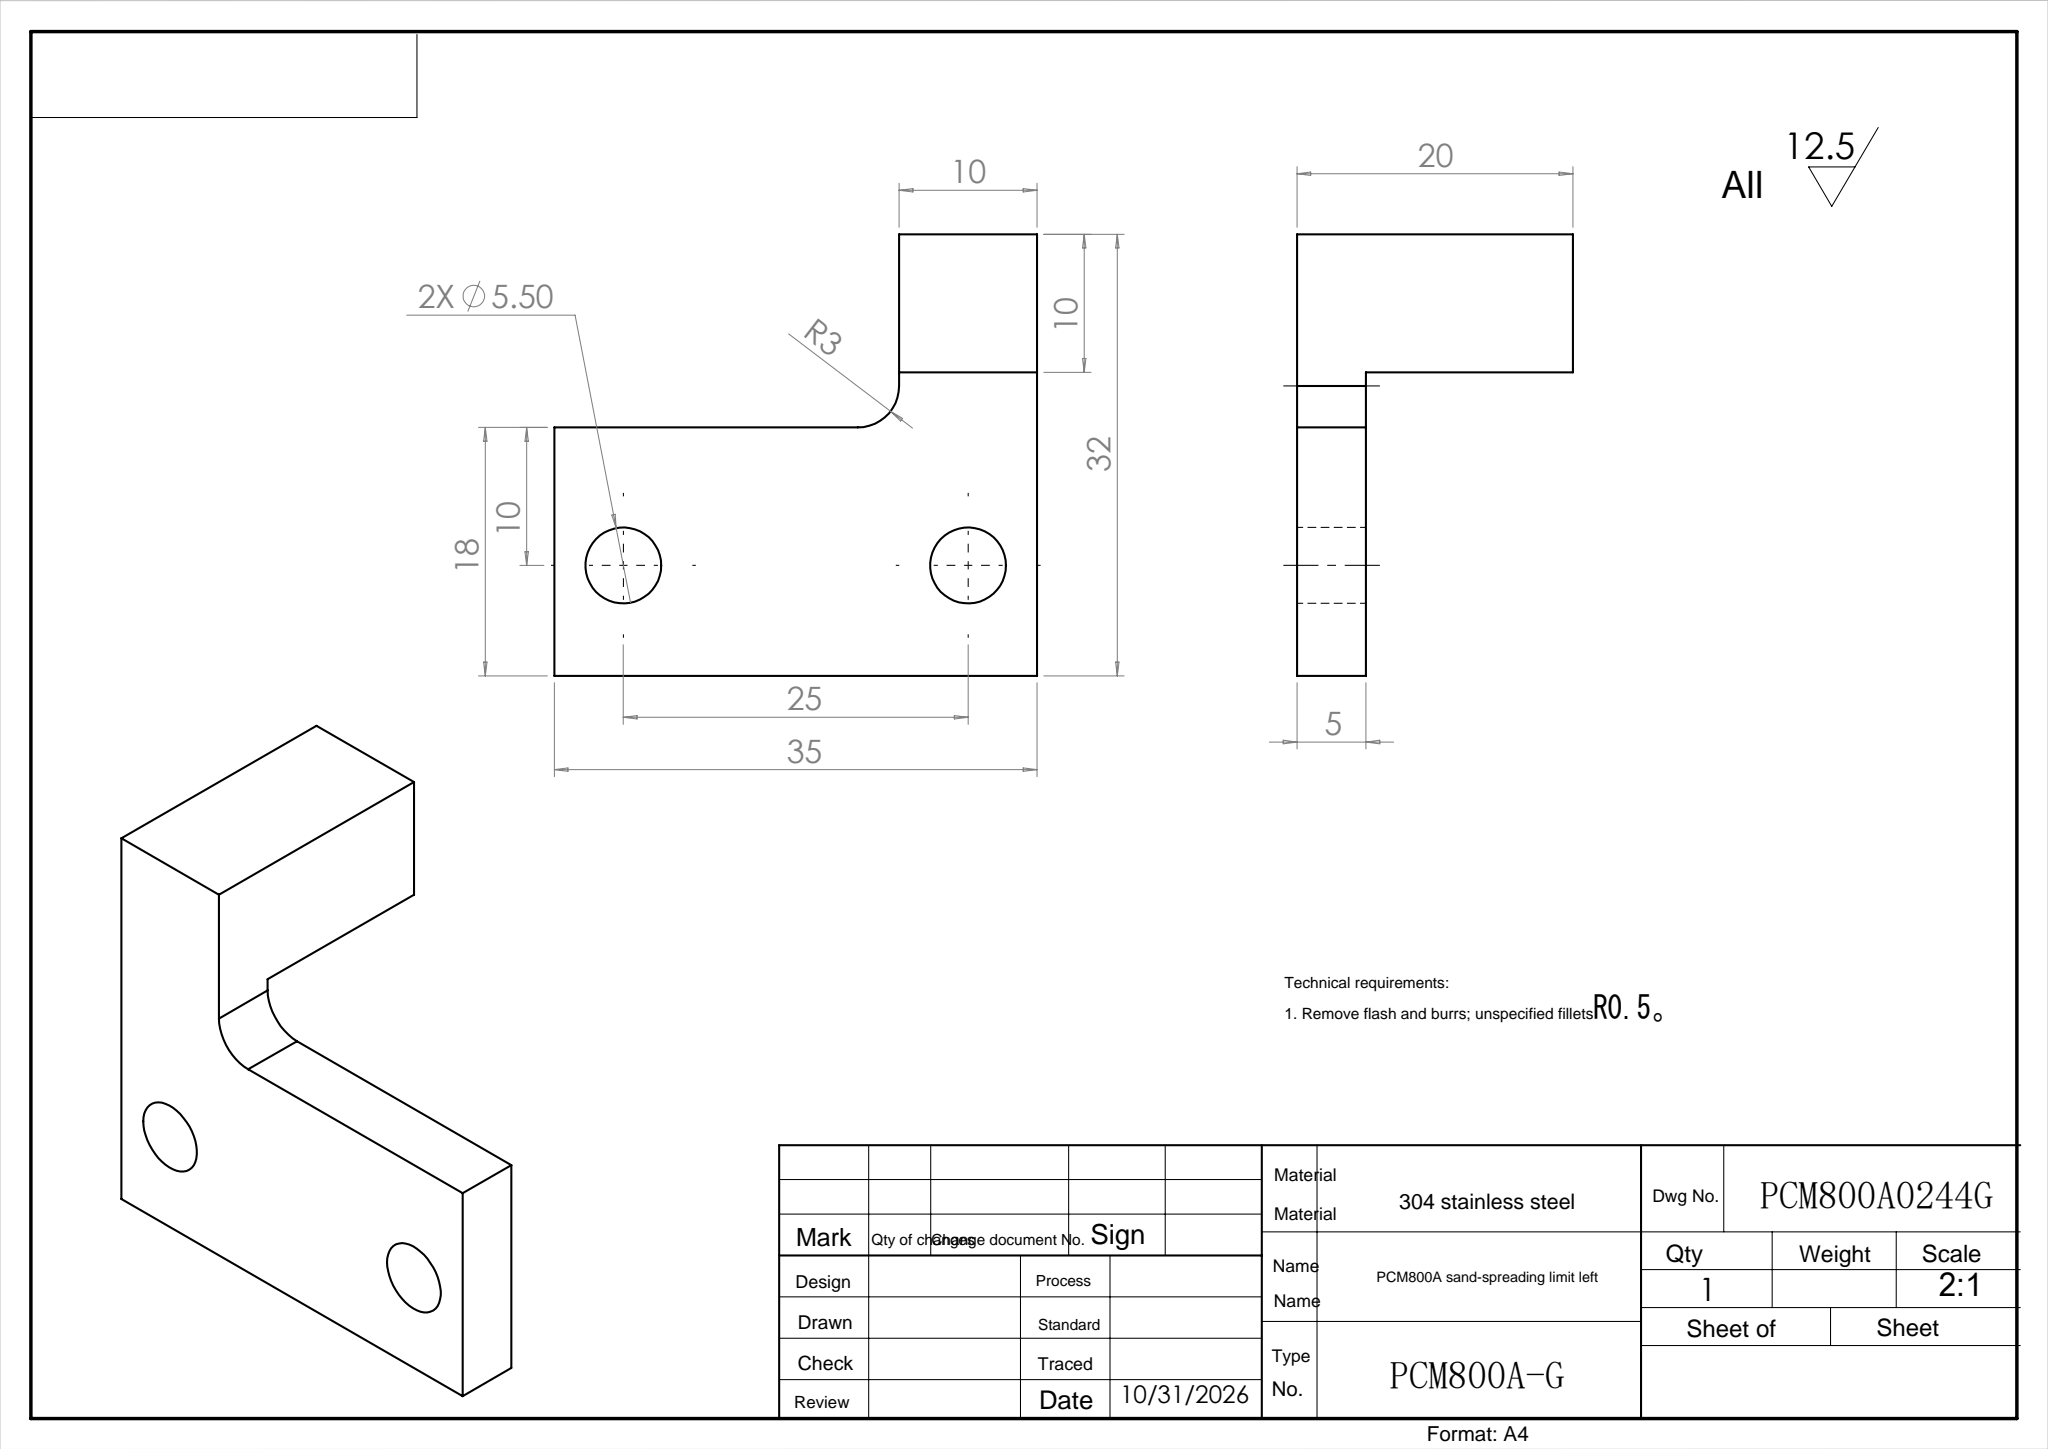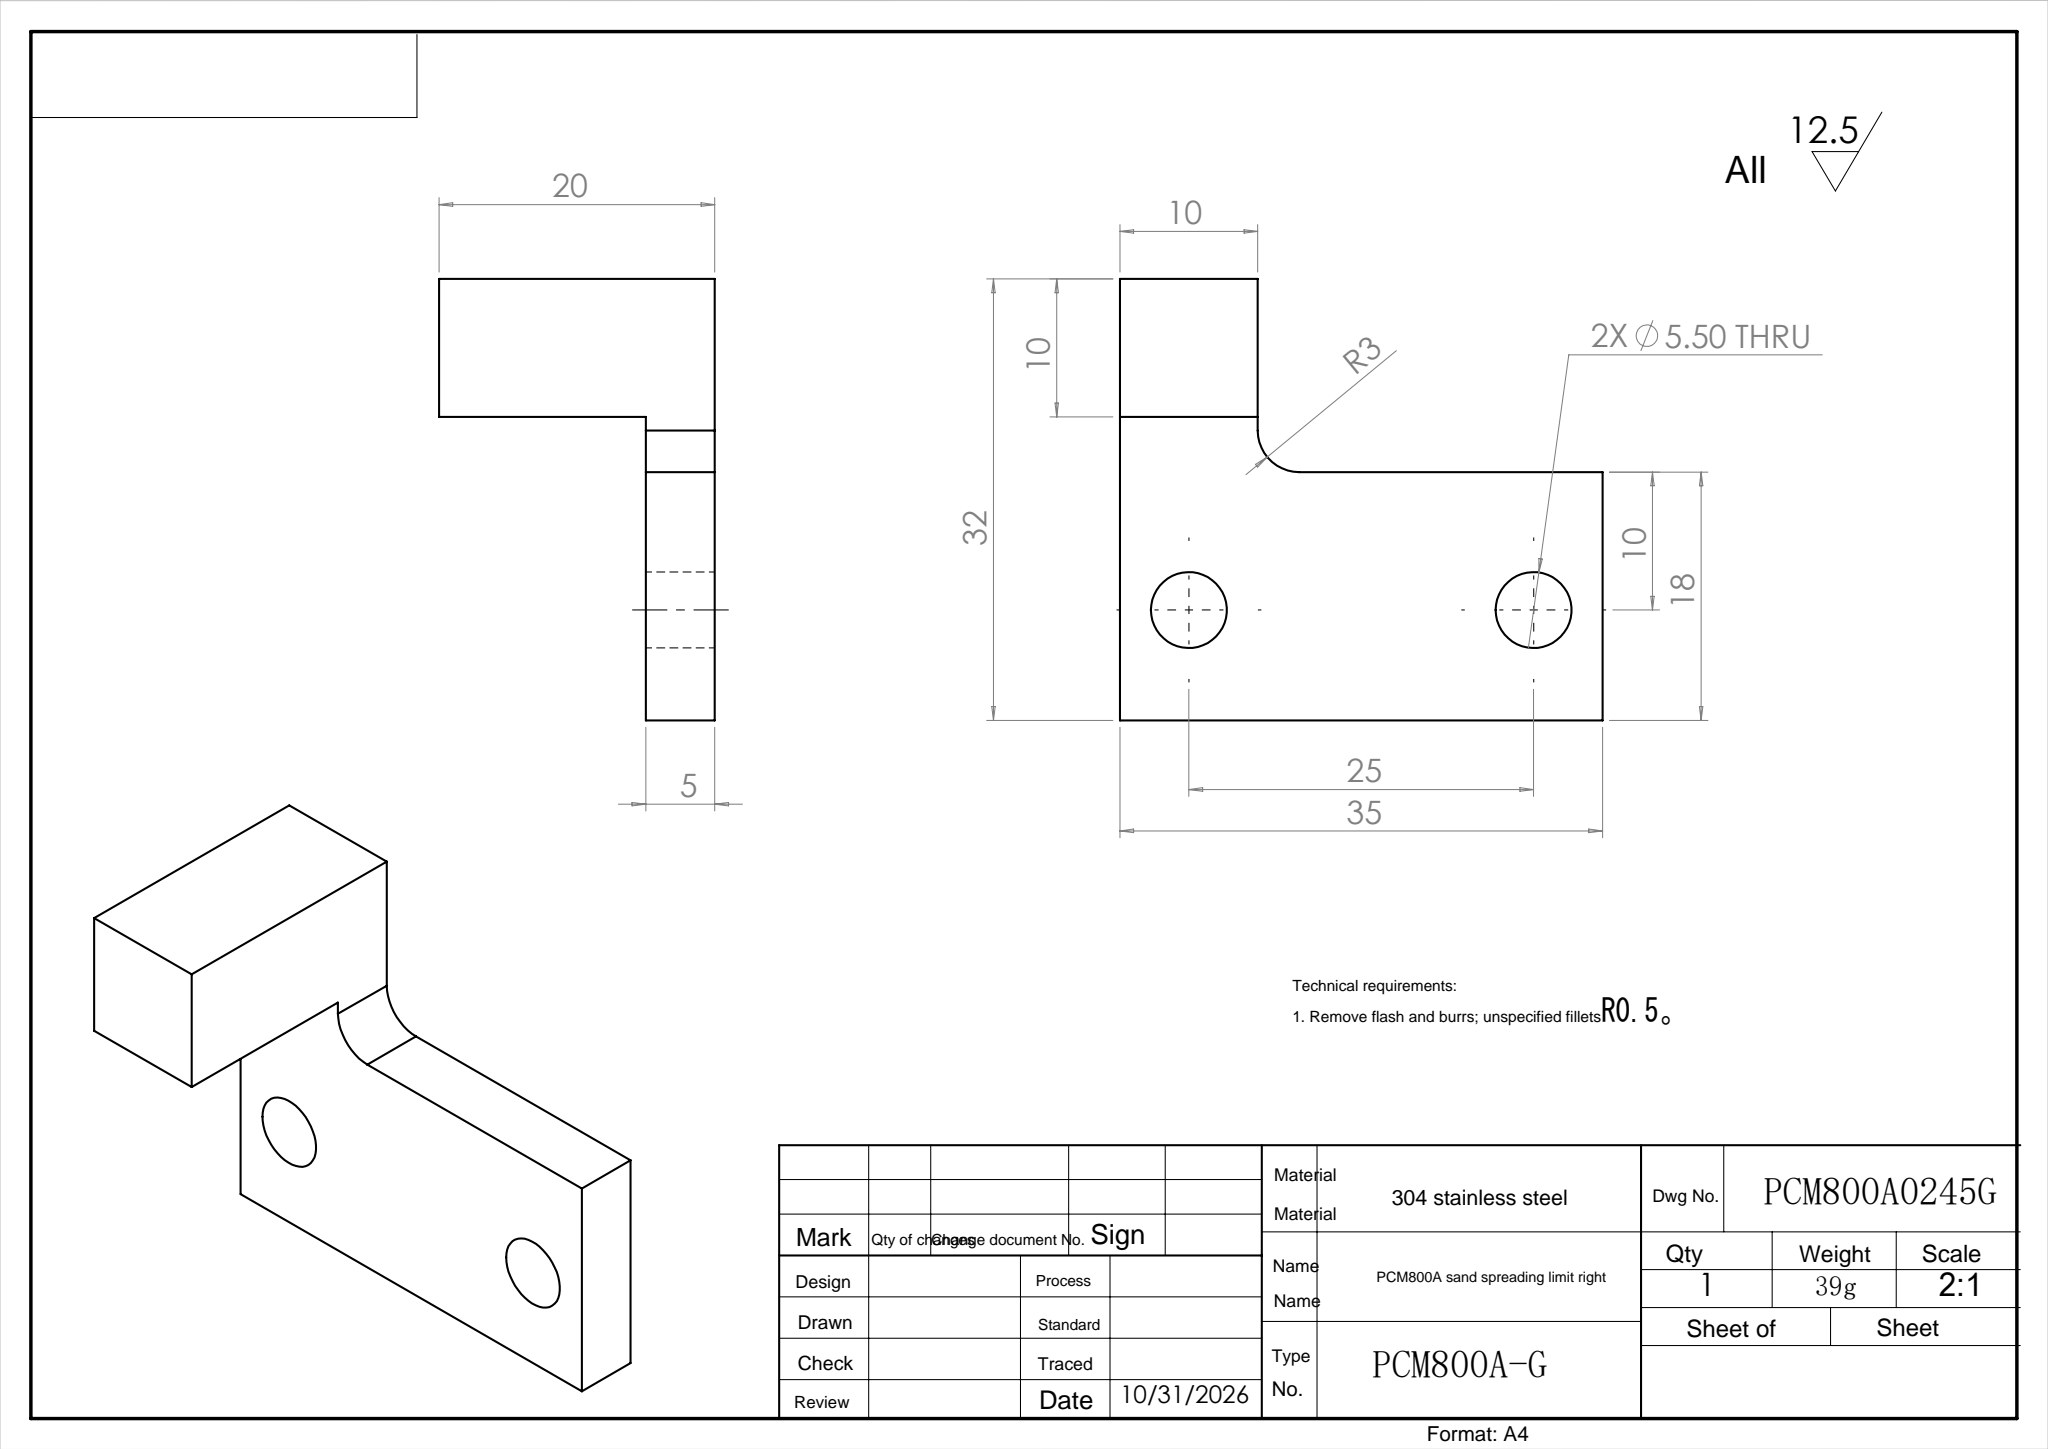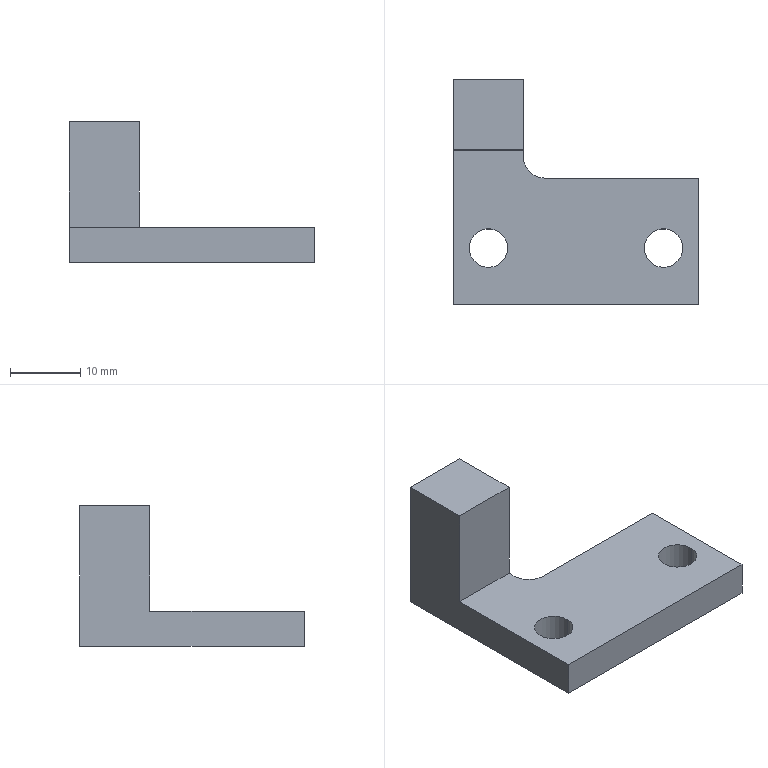Part | SolidWorks | features ICE 2, Extrusion 1 | 1 solid | 15 faces | box 35 x 32 x 20 mm | volume 5122 mm3 | plane 10 | cylinder 5 | commonest cylinder face diameters 5.5 x4 6 x1
STEP:
#1=CARTESIAN_POINT('',(7.75,8.,5.));
#2=VERTEX_POINT('',#1);
#3=CARTESIAN_POINT('',(2.25,8.,5.));
#4=VERTEX_POINT('',#3);
#5=CARTESIAN_POINT('',(5.,8.,5.));
#6=DIRECTION('',(0.,0.,-1.));
#7=DIRECTION('',(-1.,0.,0.));
#8=AXIS2_PLACEMENT_3D('',#5,#6,#7);
#9=CIRCLE('',#8,2.75);
#10=EDGE_CURVE('',#2,#4,#9,.T.);
#11=ORIENTED_EDGE('',*,*,#10,.F.);
#12=CARTESIAN_POINT('',(7.75,8.,0.));
#13=VERTEX_POINT('',#12);
#14=CARTESIAN_POINT('',(7.75,8.,20.));
#15=DIRECTION('',(0.,0.,-1.));
#16=VECTOR('',#15,1000.);
#17=LINE('',#14,#16);
#18=EDGE_CURVE('',#2,#13,#17,.T.);
#19=ORIENTED_EDGE('',*,*,#18,.T.);
#20=CARTESIAN_POINT('',(2.25,8.,0.));
#21=VERTEX_POINT('',#20);
#22=CARTESIAN_POINT('',(5.,8.,0.));
#23=DIRECTION('',(0.,0.,-1.));
#24=DIRECTION('',(-1.,0.,0.));
#25=AXIS2_PLACEMENT_3D('',#22,#23,#24);
#26=CIRCLE('',#25,2.75);
#27=EDGE_CURVE('',#13,#21,#26,.T.);
#28=ORIENTED_EDGE('',*,*,#27,.T.);
#29=CARTESIAN_POINT('',(2.25,8.,20.));
#30=DIRECTION('',(0.,0.,-1.));
#31=VECTOR('',#30,1000.);
#32=LINE('',#29,#31);
#33=EDGE_CURVE('',#4,#21,#32,.T.);
#34=ORIENTED_EDGE('',*,*,#33,.F.);
#35=EDGE_LOOP('',(#11,#19,#28,#34));
#36=FACE_OUTER_BOUND('',#35,.T.);
#37=CARTESIAN_POINT('',(5.,8.,20.));
#38=DIRECTION('',(0.,0.,-1.));
#39=DIRECTION('',(-1.,0.,0.));
#40=AXIS2_PLACEMENT_3D('',#37,#38,#39);
#41=CYLINDRICAL_SURFACE('',#40,2.75);
#42=ADVANCED_FACE('',(#36),#41,.F.);
#43=CARTESIAN_POINT('',(32.75,8.,5.));
#44=VERTEX_POINT('',#43);
#45=CARTESIAN_POINT('',(27.25,8.,5.));
#46=VERTEX_POINT('',#45);
#47=CARTESIAN_POINT('',(30.,8.,5.));
#48=DIRECTION('',(0.,0.,-1.));
#49=DIRECTION('',(-1.,0.,0.));
#50=AXIS2_PLACEMENT_3D('',#47,#48,#49);
#51=CIRCLE('',#50,2.75);
#52=EDGE_CURVE('',#44,#46,#51,.T.);
#53=ORIENTED_EDGE('',*,*,#52,.F.);
#54=CARTESIAN_POINT('',(32.75,8.,0.));
#55=VERTEX_POINT('',#54);
#56=CARTESIAN_POINT('',(32.75,8.,20.));
#57=DIRECTION('',(0.,0.,-1.));
#58=VECTOR('',#57,1000.);
#59=LINE('',#56,#58);
#60=EDGE_CURVE('',#44,#55,#59,.T.);
#61=ORIENTED_EDGE('',*,*,#60,.T.);
#62=CARTESIAN_POINT('',(27.25,8.,0.));
#63=VERTEX_POINT('',#62);
#64=CARTESIAN_POINT('',(30.,8.,0.));
#65=DIRECTION('',(0.,0.,-1.));
#66=DIRECTION('',(-1.,0.,0.));
#67=AXIS2_PLACEMENT_3D('',#64,#65,#66);
#68=CIRCLE('',#67,2.75);
#69=EDGE_CURVE('',#55,#63,#68,.T.);
#70=ORIENTED_EDGE('',*,*,#69,.T.);
#71=CARTESIAN_POINT('',(27.25,8.,20.));
#72=DIRECTION('',(0.,0.,-1.));
#73=VECTOR('',#72,1000.);
#74=LINE('',#71,#73);
#75=EDGE_CURVE('',#46,#63,#74,.T.);
#76=ORIENTED_EDGE('',*,*,#75,.F.);
#77=EDGE_LOOP('',(#53,#61,#70,#76));
#78=FACE_OUTER_BOUND('',#77,.T.);
#79=CARTESIAN_POINT('',(30.,8.,20.));
#80=DIRECTION('',(0.,0.,-1.));
#81=DIRECTION('',(-1.,0.,0.));
#82=AXIS2_PLACEMENT_3D('',#79,#80,#81);
#83=CYLINDRICAL_SURFACE('',#82,2.75);
#84=ADVANCED_FACE('',(#78),#83,.F.);
#85=CARTESIAN_POINT('',(0.,32.,0.));
#86=VERTEX_POINT('',#85);
#87=CARTESIAN_POINT('',(0.,0.,0.));
#88=VERTEX_POINT('',#87);
#89=CARTESIAN_POINT('',(0.,0.,0.));
#90=DIRECTION('',(0.,-1.,0.));
#91=VECTOR('',#90,1000.);
#92=LINE('',#89,#91);
#93=EDGE_CURVE('',#86,#88,#92,.T.);
#94=ORIENTED_EDGE('',*,*,#93,.T.);
#95=CARTESIAN_POINT('',(0.,0.,5.));
#96=VERTEX_POINT('',#95);
#97=CARTESIAN_POINT('',(0.,0.,5.));
#98=DIRECTION('',(0.,0.,-1.));
#99=VECTOR('',#98,1000.);
#100=LINE('',#97,#99);
#101=EDGE_CURVE('',#96,#88,#100,.T.);
#102=ORIENTED_EDGE('',*,*,#101,.F.);
#103=CARTESIAN_POINT('',(0.,22.,5.));
#104=VERTEX_POINT('',#103);
#105=CARTESIAN_POINT('',(0.,0.,5.));
#106=DIRECTION('',(0.,-1.,0.));
#107=VECTOR('',#106,1000.);
#108=LINE('',#105,#107);
#109=EDGE_CURVE('',#104,#96,#108,.T.);
#110=ORIENTED_EDGE('',*,*,#109,.F.);
#111=CARTESIAN_POINT('',(0.,22.,20.));
#112=VERTEX_POINT('',#111);
#113=CARTESIAN_POINT('',(0.,22.,20.));
#114=DIRECTION('',(0.,0.,-1.));
#115=VECTOR('',#114,1000.);
#116=LINE('',#113,#115);
#117=EDGE_CURVE('',#112,#104,#116,.T.);
#118=ORIENTED_EDGE('',*,*,#117,.F.);
#119=CARTESIAN_POINT('',(0.,32.,20.));
#120=VERTEX_POINT('',#119);
#121=CARTESIAN_POINT('',(0.,22.,20.));
#122=DIRECTION('',(0.,1.,0.));
#123=VECTOR('',#122,1000.);
#124=LINE('',#121,#123);
#125=EDGE_CURVE('',#112,#120,#124,.T.);
#126=ORIENTED_EDGE('',*,*,#125,.T.);
#127=CARTESIAN_POINT('',(0.,32.,20.));
#128=DIRECTION('',(0.,0.,-1.));
#129=VECTOR('',#128,1000.);
#130=LINE('',#127,#129);
#131=EDGE_CURVE('',#120,#86,#130,.T.);
#132=ORIENTED_EDGE('',*,*,#131,.T.);
#133=EDGE_LOOP('',(#94,#102,#110,#118,#126,#132));
#134=FACE_OUTER_BOUND('',#133,.T.);
#135=CARTESIAN_POINT('',(0.,0.,5.));
#136=DIRECTION('',(1.,0.,0.));
#137=DIRECTION('',(0.,0.,-1.));
#138=AXIS2_PLACEMENT_3D('',#135,#136,#137);
#139=PLANE('',#138);
#140=ADVANCED_FACE('',(#134),#139,.F.);
#141=CARTESIAN_POINT('',(35.,0.,0.));
#142=VERTEX_POINT('',#141);
#143=CARTESIAN_POINT('',(0.,0.,0.));
#144=DIRECTION('',(1.,0.,0.));
#145=VECTOR('',#144,1000.);
#146=LINE('',#143,#145);
#147=EDGE_CURVE('',#88,#142,#146,.T.);
#148=ORIENTED_EDGE('',*,*,#147,.T.);
#149=CARTESIAN_POINT('',(35.,0.,5.));
#150=VERTEX_POINT('',#149);
#151=CARTESIAN_POINT('',(35.,0.,5.));
#152=DIRECTION('',(0.,0.,-1.));
#153=VECTOR('',#152,1000.);
#154=LINE('',#151,#153);
#155=EDGE_CURVE('',#150,#142,#154,.T.);
#156=ORIENTED_EDGE('',*,*,#155,.F.);
#157=CARTESIAN_POINT('',(0.,0.,5.));
#158=DIRECTION('',(1.,0.,0.));
#159=VECTOR('',#158,1000.);
#160=LINE('',#157,#159);
#161=EDGE_CURVE('',#96,#150,#160,.T.);
#162=ORIENTED_EDGE('',*,*,#161,.F.);
#163=ORIENTED_EDGE('',*,*,#101,.T.);
#164=EDGE_LOOP('',(#148,#156,#162,#163));
#165=FACE_OUTER_BOUND('',#164,.T.);
#166=CARTESIAN_POINT('',(0.,0.,5.));
#167=DIRECTION('',(0.,1.,0.));
#168=DIRECTION('',(0.,0.,1.));
#169=AXIS2_PLACEMENT_3D('',#166,#167,#168);
#170=PLANE('',#169);
#171=ADVANCED_FACE('',(#165),#170,.F.);
#172=CARTESIAN_POINT('',(35.,18.,0.));
#173=VERTEX_POINT('',#172);
#174=CARTESIAN_POINT('',(35.,0.,0.));
#175=DIRECTION('',(0.,1.,0.));
#176=VECTOR('',#175,1000.);
#177=LINE('',#174,#176);
#178=EDGE_CURVE('',#142,#173,#177,.T.);
#179=ORIENTED_EDGE('',*,*,#178,.T.);
#180=CARTESIAN_POINT('',(35.,18.,5.));
#181=VERTEX_POINT('',#180);
#182=CARTESIAN_POINT('',(35.,18.,5.));
#183=DIRECTION('',(0.,0.,-1.));
#184=VECTOR('',#183,1000.);
#185=LINE('',#182,#184);
#186=EDGE_CURVE('',#181,#173,#185,.T.);
#187=ORIENTED_EDGE('',*,*,#186,.F.);
#188=CARTESIAN_POINT('',(35.,0.,5.));
#189=DIRECTION('',(0.,1.,0.));
#190=VECTOR('',#189,1000.);
#191=LINE('',#188,#190);
#192=EDGE_CURVE('',#150,#181,#191,.T.);
#193=ORIENTED_EDGE('',*,*,#192,.F.);
#194=ORIENTED_EDGE('',*,*,#155,.T.);
#195=EDGE_LOOP('',(#179,#187,#193,#194));
#196=FACE_OUTER_BOUND('',#195,.T.);
#197=CARTESIAN_POINT('',(35.,0.,5.));
#198=DIRECTION('',(-1.,0.,0.));
#199=DIRECTION('',(0.,0.,1.));
#200=AXIS2_PLACEMENT_3D('',#197,#198,#199);
#201=PLANE('',#200);
#202=ADVANCED_FACE('',(#196),#201,.F.);
#203=CARTESIAN_POINT('',(13.,18.,0.));
#204=VERTEX_POINT('',#203);
#205=CARTESIAN_POINT('',(13.,18.,0.));
#206=DIRECTION('',(-1.,0.,0.));
#207=VECTOR('',#206,1000.);
#208=LINE('',#205,#207);
#209=EDGE_CURVE('',#173,#204,#208,.T.);
#210=ORIENTED_EDGE('',*,*,#209,.T.);
#211=CARTESIAN_POINT('',(13.,18.,5.));
#212=VERTEX_POINT('',#211);
#213=CARTESIAN_POINT('',(13.,18.,5.));
#214=DIRECTION('',(0.,0.,-1.));
#215=VECTOR('',#214,1000.);
#216=LINE('',#213,#215);
#217=EDGE_CURVE('',#212,#204,#216,.T.);
#218=ORIENTED_EDGE('',*,*,#217,.F.);
#219=CARTESIAN_POINT('',(13.,18.,5.));
#220=DIRECTION('',(-1.,0.,0.));
#221=VECTOR('',#220,1000.);
#222=LINE('',#219,#221);
#223=EDGE_CURVE('',#181,#212,#222,.T.);
#224=ORIENTED_EDGE('',*,*,#223,.F.);
#225=ORIENTED_EDGE('',*,*,#186,.T.);
#226=EDGE_LOOP('',(#210,#218,#224,#225));
#227=FACE_OUTER_BOUND('',#226,.T.);
#228=CARTESIAN_POINT('',(13.,18.,5.));
#229=DIRECTION('',(0.,-1.,0.));
#230=DIRECTION('',(0.,0.,-1.));
#231=AXIS2_PLACEMENT_3D('',#228,#229,#230);
#232=PLANE('',#231);
#233=ADVANCED_FACE('',(#227),#232,.F.);
#234=CARTESIAN_POINT('',(10.,21.,0.));
#235=VERTEX_POINT('',#234);
#236=CARTESIAN_POINT('',(13.,21.,0.));
#237=DIRECTION('',(0.,0.,-1.));
#238=DIRECTION('',(-1.,0.,0.));
#239=AXIS2_PLACEMENT_3D('',#236,#237,#238);
#240=CIRCLE('',#239,3.);
#241=EDGE_CURVE('',#204,#235,#240,.T.);
#242=ORIENTED_EDGE('',*,*,#241,.T.);
#243=CARTESIAN_POINT('',(10.,21.,5.));
#244=VERTEX_POINT('',#243);
#245=CARTESIAN_POINT('',(10.,21.,5.));
#246=DIRECTION('',(0.,0.,-1.));
#247=VECTOR('',#246,1000.);
#248=LINE('',#245,#247);
#249=EDGE_CURVE('',#244,#235,#248,.T.);
#250=ORIENTED_EDGE('',*,*,#249,.F.);
#251=CARTESIAN_POINT('',(13.,21.,5.));
#252=DIRECTION('',(0.,0.,-1.));
#253=DIRECTION('',(-1.,0.,0.));
#254=AXIS2_PLACEMENT_3D('',#251,#252,#253);
#255=CIRCLE('',#254,3.);
#256=EDGE_CURVE('',#212,#244,#255,.T.);
#257=ORIENTED_EDGE('',*,*,#256,.F.);
#258=ORIENTED_EDGE('',*,*,#217,.T.);
#259=EDGE_LOOP('',(#242,#250,#257,#258));
#260=FACE_OUTER_BOUND('',#259,.T.);
#261=CARTESIAN_POINT('',(13.,21.,5.));
#262=DIRECTION('',(0.,0.,-1.));
#263=DIRECTION('',(-1.,0.,0.));
#264=AXIS2_PLACEMENT_3D('',#261,#262,#263);
#265=CYLINDRICAL_SURFACE('',#264,3.);
#266=ADVANCED_FACE('',(#260),#265,.F.);
#267=CARTESIAN_POINT('',(10.,32.,0.));
#268=VERTEX_POINT('',#267);
#269=CARTESIAN_POINT('',(10.,21.,0.));
#270=DIRECTION('',(0.,1.,0.));
#271=VECTOR('',#270,1000.);
#272=LINE('',#269,#271);
#273=EDGE_CURVE('',#235,#268,#272,.T.);
#274=ORIENTED_EDGE('',*,*,#273,.T.);
#275=CARTESIAN_POINT('',(10.,32.,20.));
#276=VERTEX_POINT('',#275);
#277=CARTESIAN_POINT('',(10.,32.,20.));
#278=DIRECTION('',(0.,0.,-1.));
#279=VECTOR('',#278,1000.);
#280=LINE('',#277,#279);
#281=EDGE_CURVE('',#276,#268,#280,.T.);
#282=ORIENTED_EDGE('',*,*,#281,.F.);
#283=CARTESIAN_POINT('',(10.,22.,20.));
#284=VERTEX_POINT('',#283);
#285=CARTESIAN_POINT('',(10.,22.,20.));
#286=DIRECTION('',(0.,-1.,0.));
#287=VECTOR('',#286,1000.);
#288=LINE('',#285,#287);
#289=EDGE_CURVE('',#276,#284,#288,.T.);
#290=ORIENTED_EDGE('',*,*,#289,.T.);
#291=CARTESIAN_POINT('',(10.,22.,5.));
#292=VERTEX_POINT('',#291);
#293=CARTESIAN_POINT('',(10.,22.,20.));
#294=DIRECTION('',(0.,0.,-1.));
#295=VECTOR('',#294,1000.);
#296=LINE('',#293,#295);
#297=EDGE_CURVE('',#284,#292,#296,.T.);
#298=ORIENTED_EDGE('',*,*,#297,.T.);
#299=CARTESIAN_POINT('',(10.,21.,5.));
#300=DIRECTION('',(0.,1.,0.));
#301=VECTOR('',#300,1000.);
#302=LINE('',#299,#301);
#303=EDGE_CURVE('',#244,#292,#302,.T.);
#304=ORIENTED_EDGE('',*,*,#303,.F.);
#305=ORIENTED_EDGE('',*,*,#249,.T.);
#306=EDGE_LOOP('',(#274,#282,#290,#298,#304,#305));
#307=FACE_OUTER_BOUND('',#306,.T.);
#308=CARTESIAN_POINT('',(10.,21.,5.));
#309=DIRECTION('',(-1.,0.,0.));
#310=DIRECTION('',(0.,-1.,0.));
#311=AXIS2_PLACEMENT_3D('',#308,#309,#310);
#312=PLANE('',#311);
#313=ADVANCED_FACE('',(#307),#312,.F.);
#314=CARTESIAN_POINT('',(5.,8.,5.));
#315=DIRECTION('',(0.,0.,-1.));
#316=DIRECTION('',(-1.,0.,0.));
#317=AXIS2_PLACEMENT_3D('',#314,#315,#316);
#318=CIRCLE('',#317,2.75);
#319=EDGE_CURVE('',#4,#2,#318,.T.);
#320=ORIENTED_EDGE('',*,*,#319,.T.);
#321=ORIENTED_EDGE('',*,*,#10,.T.);
#322=EDGE_LOOP('',(#320,#321));
#323=FACE_BOUND('',#322,.T.);
#324=CARTESIAN_POINT('',(30.,8.,5.));
#325=DIRECTION('',(0.,0.,-1.));
#326=DIRECTION('',(-1.,0.,0.));
#327=AXIS2_PLACEMENT_3D('',#324,#325,#326);
#328=CIRCLE('',#327,2.75);
#329=EDGE_CURVE('',#46,#44,#328,.T.);
#330=ORIENTED_EDGE('',*,*,#329,.T.);
#331=ORIENTED_EDGE('',*,*,#52,.T.);
#332=EDGE_LOOP('',(#330,#331));
#333=FACE_BOUND('',#332,.T.);
#334=ORIENTED_EDGE('',*,*,#109,.T.);
#335=ORIENTED_EDGE('',*,*,#161,.T.);
#336=ORIENTED_EDGE('',*,*,#192,.T.);
#337=ORIENTED_EDGE('',*,*,#223,.T.);
#338=ORIENTED_EDGE('',*,*,#256,.T.);
#339=ORIENTED_EDGE('',*,*,#303,.T.);
#340=CARTESIAN_POINT('',(0.,22.,5.));
#341=DIRECTION('',(-1.,0.,0.));
#342=VECTOR('',#341,1000.);
#343=LINE('',#340,#342);
#344=EDGE_CURVE('',#292,#104,#343,.T.);
#345=ORIENTED_EDGE('',*,*,#344,.T.);
#346=EDGE_LOOP('',(#334,#335,#336,#337,#338,#339,#345));
#347=FACE_OUTER_BOUND('',#346,.T.);
#348=CARTESIAN_POINT('',(13.,21.,5.));
#349=DIRECTION('',(0.,0.,-1.));
#350=DIRECTION('',(-1.,0.,0.));
#351=AXIS2_PLACEMENT_3D('',#348,#349,#350);
#352=PLANE('',#351);
#353=ADVANCED_FACE('',(#323,#333,#347),#352,.F.);
#354=CARTESIAN_POINT('',(5.,8.,0.));
#355=DIRECTION('',(0.,0.,-1.));
#356=DIRECTION('',(-1.,0.,0.));
#357=AXIS2_PLACEMENT_3D('',#354,#355,#356);
#358=CIRCLE('',#357,2.75);
#359=EDGE_CURVE('',#21,#13,#358,.T.);
#360=ORIENTED_EDGE('',*,*,#359,.F.);
#361=ORIENTED_EDGE('',*,*,#27,.F.);
#362=EDGE_LOOP('',(#360,#361));
#363=FACE_BOUND('',#362,.T.);
#364=CARTESIAN_POINT('',(30.,8.,0.));
#365=DIRECTION('',(0.,0.,-1.));
#366=DIRECTION('',(-1.,0.,0.));
#367=AXIS2_PLACEMENT_3D('',#364,#365,#366);
#368=CIRCLE('',#367,2.75);
#369=EDGE_CURVE('',#63,#55,#368,.T.);
#370=ORIENTED_EDGE('',*,*,#369,.F.);
#371=ORIENTED_EDGE('',*,*,#69,.F.);
#372=EDGE_LOOP('',(#370,#371));
#373=FACE_BOUND('',#372,.T.);
#374=ORIENTED_EDGE('',*,*,#93,.F.);
#375=CARTESIAN_POINT('',(0.,32.,0.));
#376=DIRECTION('',(1.,0.,0.));
#377=VECTOR('',#376,1000.);
#378=LINE('',#375,#377);
#379=EDGE_CURVE('',#86,#268,#378,.T.);
#380=ORIENTED_EDGE('',*,*,#379,.T.);
#381=ORIENTED_EDGE('',*,*,#273,.F.);
#382=ORIENTED_EDGE('',*,*,#241,.F.);
#383=ORIENTED_EDGE('',*,*,#209,.F.);
#384=ORIENTED_EDGE('',*,*,#178,.F.);
#385=ORIENTED_EDGE('',*,*,#147,.F.);
#386=EDGE_LOOP('',(#374,#380,#381,#382,#383,#384,#385));
#387=FACE_OUTER_BOUND('',#386,.T.);
#388=CARTESIAN_POINT('',(13.,21.,0.));
#389=DIRECTION('',(0.,0.,-1.));
#390=DIRECTION('',(-1.,0.,0.));
#391=AXIS2_PLACEMENT_3D('',#388,#389,#390);
#392=PLANE('',#391);
#393=ADVANCED_FACE('',(#363,#373,#387),#392,.T.);
#394=ORIENTED_EDGE('',*,*,#344,.F.);
#395=ORIENTED_EDGE('',*,*,#297,.F.);
#396=CARTESIAN_POINT('',(0.,22.,20.));
#397=DIRECTION('',(-1.,0.,0.));
#398=VECTOR('',#397,1000.);
#399=LINE('',#396,#398);
#400=EDGE_CURVE('',#284,#112,#399,.T.);
#401=ORIENTED_EDGE('',*,*,#400,.T.);
#402=ORIENTED_EDGE('',*,*,#117,.T.);
#403=EDGE_LOOP('',(#394,#395,#401,#402));
#404=FACE_OUTER_BOUND('',#403,.T.);
#405=CARTESIAN_POINT('',(0.,22.,20.));
#406=DIRECTION('',(0.,-1.,0.));
#407=DIRECTION('',(0.,0.,-1.));
#408=AXIS2_PLACEMENT_3D('',#405,#406,#407);
#409=PLANE('',#408);
#410=ADVANCED_FACE('',(#404),#409,.T.);
#411=ORIENTED_EDGE('',*,*,#379,.F.);
#412=ORIENTED_EDGE('',*,*,#131,.F.);
#413=CARTESIAN_POINT('',(0.,32.,20.));
#414=DIRECTION('',(1.,0.,0.));
#415=VECTOR('',#414,1000.);
#416=LINE('',#413,#415);
#417=EDGE_CURVE('',#120,#276,#416,.T.);
#418=ORIENTED_EDGE('',*,*,#417,.T.);
#419=ORIENTED_EDGE('',*,*,#281,.T.);
#420=EDGE_LOOP('',(#411,#412,#418,#419));
#421=FACE_OUTER_BOUND('',#420,.T.);
#422=CARTESIAN_POINT('',(0.,32.,20.));
#423=DIRECTION('',(0.,1.,0.));
#424=DIRECTION('',(0.,0.,1.));
#425=AXIS2_PLACEMENT_3D('',#422,#423,#424);
#426=PLANE('',#425);
#427=ADVANCED_FACE('',(#421),#426,.T.);
#428=ORIENTED_EDGE('',*,*,#125,.F.);
#429=ORIENTED_EDGE('',*,*,#400,.F.);
#430=ORIENTED_EDGE('',*,*,#289,.F.);
#431=ORIENTED_EDGE('',*,*,#417,.F.);
#432=EDGE_LOOP('',(#428,#429,#430,#431));
#433=FACE_OUTER_BOUND('',#432,.T.);
#434=CARTESIAN_POINT('',(0.,32.,20.));
#435=DIRECTION('',(0.,0.,-1.));
#436=DIRECTION('',(-1.,0.,0.));
#437=AXIS2_PLACEMENT_3D('',#434,#435,#436);
#438=PLANE('',#437);
#439=ADVANCED_FACE('',(#433),#438,.F.);
#440=ORIENTED_EDGE('',*,*,#60,.F.);
#441=ORIENTED_EDGE('',*,*,#329,.F.);
#442=ORIENTED_EDGE('',*,*,#75,.T.);
#443=ORIENTED_EDGE('',*,*,#369,.T.);
#444=EDGE_LOOP('',(#440,#441,#442,#443));
#445=FACE_OUTER_BOUND('',#444,.T.);
#446=CARTESIAN_POINT('',(30.,8.,20.));
#447=DIRECTION('',(0.,0.,-1.));
#448=DIRECTION('',(-1.,0.,0.));
#449=AXIS2_PLACEMENT_3D('',#446,#447,#448);
#450=CYLINDRICAL_SURFACE('',#449,2.75);
#451=ADVANCED_FACE('',(#445),#450,.F.);
#452=ORIENTED_EDGE('',*,*,#18,.F.);
#453=ORIENTED_EDGE('',*,*,#319,.F.);
#454=ORIENTED_EDGE('',*,*,#33,.T.);
#455=ORIENTED_EDGE('',*,*,#359,.T.);
#456=EDGE_LOOP('',(#452,#453,#454,#455));
#457=FACE_OUTER_BOUND('',#456,.T.);
#458=CARTESIAN_POINT('',(5.,8.,20.));
#459=DIRECTION('',(0.,0.,-1.));
#460=DIRECTION('',(-1.,0.,0.));
#461=AXIS2_PLACEMENT_3D('',#458,#459,#460);
#462=CYLINDRICAL_SURFACE('',#461,2.75);
#463=ADVANCED_FACE('',(#457),#462,.F.);
#464=CLOSED_SHELL('',(#42,#84,#140,#171,#202,#233,#266,#313,#353,#393,#410,#427,#439,#451,#463));
#465=MANIFOLD_SOLID_BREP('',#464);
#466=CARTESIAN_POINT('',(0.,0.,0.));
#467=DIRECTION('',(0.,0.,1.));
#468=DIRECTION('',(1.,0.,0.));
#469=AXIS2_PLACEMENT_3D('',#466,#467,#468);
#470=(LENGTH_UNIT()NAMED_UNIT(*)SI_UNIT(.MILLI.,.METRE.));
#471=UNCERTAINTY_MEASURE_WITH_UNIT(LENGTH_MEASURE(0.00001),#470,'','');
#472=(NAMED_UNIT(*)PLANE_ANGLE_UNIT()SI_UNIT($,.RADIAN.));
#473=(NAMED_UNIT(*)SI_UNIT($,.STERADIAN.)SOLID_ANGLE_UNIT());
#474=(GEOMETRIC_REPRESENTATION_CONTEXT(3)GLOBAL_UNCERTAINTY_ASSIGNED_CONTEXT((#471))GLOBAL_UNIT_ASSIGNED_CONTEXT((#470,#472,#473))REPRESENTATION_CONTEXT('',''));
#475=ADVANCED_BREP_SHAPE_REPRESENTATION('',(#465,#469),#474);